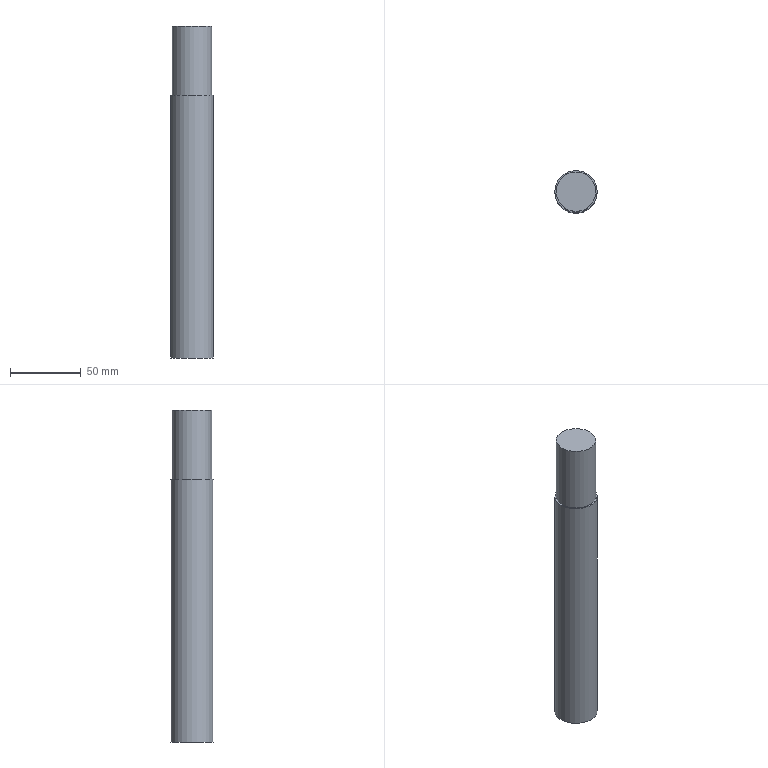Part | NX | features solid 2 | 1 solid | 5 faces | box 30 x 30 x 235 mm | volume 161648 mm3 | plane 3 | cylinder 2 | commonest cylinder face diameters 28 x1 30 x1
STEP:
#1=CARTESIAN_POINT('',(55.,-155.,-94.));
#2=VERTEX_POINT('',#1);
#3=CARTESIAN_POINT('',(70.,-155.,-94.));
#4=DIRECTION('',(0.,0.,-1.));
#5=DIRECTION('',(-1.,0.,0.));
#6=AXIS2_PLACEMENT_3D('',#3,#4,#5);
#7=CIRCLE('',#6,15.);
#8=EDGE_CURVE('',#2,#2,#7,.T.);
#9=ORIENTED_EDGE('',*,*,#8,.T.);
#10=EDGE_LOOP('',(#9));
#11=FACE_BOUND('',#10,.T.);
#12=CARTESIAN_POINT('',(55.,-155.,-280.));
#13=VERTEX_POINT('',#12);
#14=CARTESIAN_POINT('',(70.,-155.,-280.));
#15=DIRECTION('',(0.,0.,-1.));
#16=DIRECTION('',(-1.,0.,0.));
#17=AXIS2_PLACEMENT_3D('',#14,#15,#16);
#18=CIRCLE('',#17,15.);
#19=EDGE_CURVE('',#13,#13,#18,.T.);
#20=ORIENTED_EDGE('',*,*,#19,.F.);
#21=EDGE_LOOP('',(#20));
#22=FACE_BOUND('',#21,.T.);
#23=CARTESIAN_POINT('',(70.,-155.,-94.));
#24=DIRECTION('',(0.,0.,-1.));
#25=DIRECTION('',(-1.,0.,0.));
#26=AXIS2_PLACEMENT_3D('',#23,#24,#25);
#27=CYLINDRICAL_SURFACE('',#26,15.);
#28=ADVANCED_FACE('',(#11,#22),#27,.T.);
#29=CARTESIAN_POINT('',(56.,-155.,-94.));
#30=VERTEX_POINT('',#29);
#31=CARTESIAN_POINT('',(70.,-155.,-94.));
#32=DIRECTION('',(0.,0.,-1.));
#33=DIRECTION('',(-1.,0.,0.));
#34=AXIS2_PLACEMENT_3D('',#31,#32,#33);
#35=CIRCLE('',#34,14.);
#36=EDGE_CURVE('',#30,#30,#35,.T.);
#37=ORIENTED_EDGE('',*,*,#36,.T.);
#38=EDGE_LOOP('',(#37));
#39=FACE_BOUND('',#38,.T.);
#40=ORIENTED_EDGE('',*,*,#8,.F.);
#41=EDGE_LOOP('',(#40));
#42=FACE_BOUND('',#41,.T.);
#43=CARTESIAN_POINT('',(70.,-155.,-94.));
#44=DIRECTION('',(0.,0.,-1.));
#45=DIRECTION('',(-1.,0.,0.));
#46=AXIS2_PLACEMENT_3D('',#43,#44,#45);
#47=PLANE('',#46);
#48=ADVANCED_FACE('',(#39,#42),#47,.F.);
#49=ORIENTED_EDGE('',*,*,#19,.T.);
#50=EDGE_LOOP('',(#49));
#51=FACE_BOUND('',#50,.T.);
#52=CARTESIAN_POINT('',(70.,-155.,-280.));
#53=DIRECTION('',(0.,0.,-1.));
#54=DIRECTION('',(-1.,0.,0.));
#55=AXIS2_PLACEMENT_3D('',#52,#53,#54);
#56=PLANE('',#55);
#57=ADVANCED_FACE('',(#51),#56,.T.);
#58=CARTESIAN_POINT('',(56.,-155.,-45.));
#59=VERTEX_POINT('',#58);
#60=CARTESIAN_POINT('',(70.,-155.,-45.));
#61=DIRECTION('',(0.,0.,-1.));
#62=DIRECTION('',(-1.,0.,0.));
#63=AXIS2_PLACEMENT_3D('',#60,#61,#62);
#64=CIRCLE('',#63,14.);
#65=EDGE_CURVE('',#59,#59,#64,.T.);
#66=ORIENTED_EDGE('',*,*,#65,.T.);
#67=EDGE_LOOP('',(#66));
#68=FACE_BOUND('',#67,.T.);
#69=ORIENTED_EDGE('',*,*,#36,.F.);
#70=EDGE_LOOP('',(#69));
#71=FACE_BOUND('',#70,.T.);
#72=CARTESIAN_POINT('',(70.,-155.,-45.));
#73=DIRECTION('',(0.,0.,-1.));
#74=DIRECTION('',(-1.,0.,0.));
#75=AXIS2_PLACEMENT_3D('',#72,#73,#74);
#76=CYLINDRICAL_SURFACE('',#75,14.);
#77=ADVANCED_FACE('',(#68,#71),#76,.T.);
#78=ORIENTED_EDGE('',*,*,#65,.F.);
#79=EDGE_LOOP('',(#78));
#80=FACE_BOUND('',#79,.T.);
#81=CARTESIAN_POINT('',(70.,-155.,-45.));
#82=DIRECTION('',(0.,0.,-1.));
#83=DIRECTION('',(-1.,0.,0.));
#84=AXIS2_PLACEMENT_3D('',#81,#82,#83);
#85=PLANE('',#84);
#86=ADVANCED_FACE('',(#80),#85,.F.);
#87=CLOSED_SHELL('',(#28,#48,#57,#77,#86));
#88=MANIFOLD_SOLID_BREP('',#87);
#89=(LENGTH_UNIT()NAMED_UNIT(*)SI_UNIT(.MILLI.,.METRE.));
#90=UNCERTAINTY_MEASURE_WITH_UNIT(LENGTH_MEASURE(0.00001),#89,'','');
#91=(NAMED_UNIT(*)PLANE_ANGLE_UNIT()SI_UNIT($,.RADIAN.));
#92=(NAMED_UNIT(*)SI_UNIT($,.STERADIAN.)SOLID_ANGLE_UNIT());
#93=(GEOMETRIC_REPRESENTATION_CONTEXT(3)GLOBAL_UNCERTAINTY_ASSIGNED_CONTEXT((#90))GLOBAL_UNIT_ASSIGNED_CONTEXT((#89,#91,#92))REPRESENTATION_CONTEXT('',''));
#94=ADVANCED_BREP_SHAPE_REPRESENTATION('',(#88),#93);